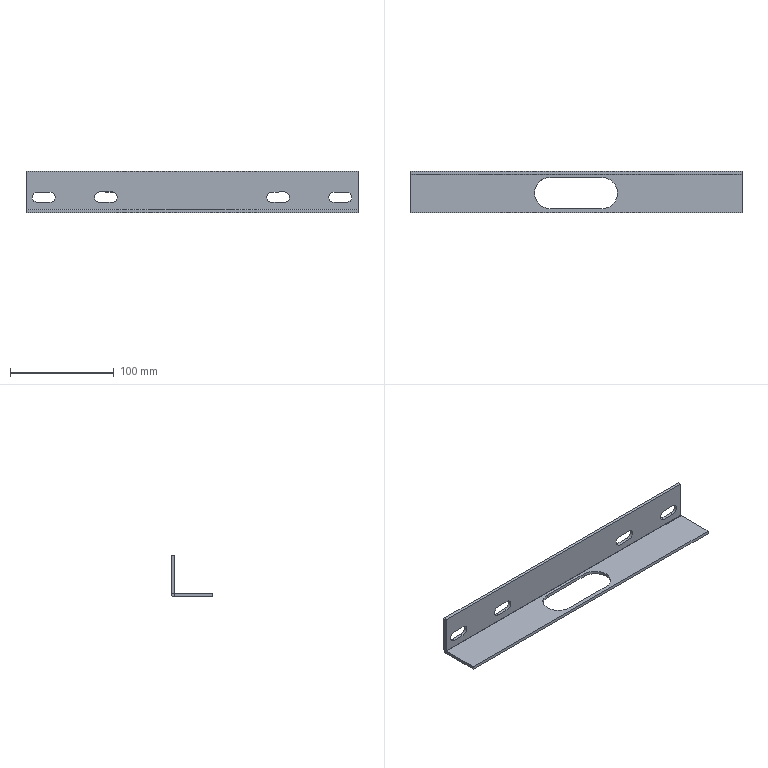Part | 1 solid | 35 faces | box 320 x 40 x 40 mm | volume 64216 mm3 | plane 22 | cylinder 13 | commonest cylinder face diameters 10 x8 30 x3 0.4 x1 6.4 x1
STEP:
#1=CARTESIAN_POINT('',(40.,-1.,-3.));
#2=VERTEX_POINT('',#1);
#3=CARTESIAN_POINT('',(25.,14.,-3.));
#4=VERTEX_POINT('',#3);
#5=CARTESIAN_POINT('',(25.,-1.,-3.));
#6=DIRECTION('',(0.,0.,1.));
#7=DIRECTION('',(1.,0.,0.));
#8=AXIS2_PLACEMENT_3D('',#5,#6,#7);
#9=CIRCLE('',#8,15.);
#10=EDGE_CURVE('',#2,#4,#9,.T.);
#11=ORIENTED_EDGE('',*,*,#10,.F.);
#12=CARTESIAN_POINT('',(40.,-1.,0.));
#13=VERTEX_POINT('',#12);
#14=CARTESIAN_POINT('',(40.,-1.,-10.));
#15=DIRECTION('',(0.,0.,1.));
#16=VECTOR('',#15,1000.);
#17=LINE('',#14,#16);
#18=EDGE_CURVE('',#2,#13,#17,.T.);
#19=ORIENTED_EDGE('',*,*,#18,.T.);
#20=CARTESIAN_POINT('',(25.,14.,0.));
#21=VERTEX_POINT('',#20);
#22=CARTESIAN_POINT('',(25.,-1.,0.));
#23=DIRECTION('',(0.,0.,1.));
#24=DIRECTION('',(1.,0.,0.));
#25=AXIS2_PLACEMENT_3D('',#22,#23,#24);
#26=CIRCLE('',#25,15.);
#27=EDGE_CURVE('',#13,#21,#26,.T.);
#28=ORIENTED_EDGE('',*,*,#27,.T.);
#29=CARTESIAN_POINT('',(25.,14.,-10.));
#30=DIRECTION('',(0.,0.,1.));
#31=VECTOR('',#30,1000.);
#32=LINE('',#29,#31);
#33=EDGE_CURVE('',#4,#21,#32,.T.);
#34=ORIENTED_EDGE('',*,*,#33,.F.);
#35=EDGE_LOOP('',(#11,#19,#28,#34));
#36=FACE_OUTER_BOUND('',#35,.T.);
#37=CARTESIAN_POINT('',(25.,-1.,-10.));
#38=DIRECTION('',(0.,0.,1.));
#39=DIRECTION('',(1.,0.,0.));
#40=AXIS2_PLACEMENT_3D('',#37,#38,#39);
#41=CYLINDRICAL_SURFACE('',#40,15.);
#42=ADVANCED_FACE('',(#36),#41,.F.);
#43=CARTESIAN_POINT('',(-160.,16.8,0.));
#44=VERTEX_POINT('',#43);
#45=CARTESIAN_POINT('',(-160.,-20.,0.));
#46=VERTEX_POINT('',#45);
#47=CARTESIAN_POINT('',(-160.,20.,0.));
#48=DIRECTION('',(0.,-1.,0.));
#49=VECTOR('',#48,1000.);
#50=LINE('',#47,#49);
#51=EDGE_CURVE('',#44,#46,#50,.T.);
#52=ORIENTED_EDGE('',*,*,#51,.F.);
#53=CARTESIAN_POINT('',(-160.,16.8,-3.));
#54=VERTEX_POINT('',#53);
#55=CARTESIAN_POINT('',(-160.,16.8,0.));
#56=DIRECTION('',(0.,0.,-1.));
#57=VECTOR('',#56,1000.);
#58=LINE('',#55,#57);
#59=EDGE_CURVE('',#44,#54,#58,.T.);
#60=ORIENTED_EDGE('',*,*,#59,.T.);
#61=CARTESIAN_POINT('',(-160.,-20.,-3.));
#62=VERTEX_POINT('',#61);
#63=CARTESIAN_POINT('',(-160.,20.,-3.));
#64=DIRECTION('',(0.,-1.,0.));
#65=VECTOR('',#64,1000.);
#66=LINE('',#63,#65);
#67=EDGE_CURVE('',#54,#62,#66,.T.);
#68=ORIENTED_EDGE('',*,*,#67,.T.);
#69=CARTESIAN_POINT('',(-160.,-20.,-3.));
#70=DIRECTION('',(0.,0.,1.));
#71=VECTOR('',#70,1000.);
#72=LINE('',#69,#71);
#73=EDGE_CURVE('',#62,#46,#72,.T.);
#74=ORIENTED_EDGE('',*,*,#73,.T.);
#75=EDGE_LOOP('',(#52,#60,#68,#74));
#76=FACE_OUTER_BOUND('',#75,.T.);
#77=CARTESIAN_POINT('',(-160.,20.,-3.));
#78=DIRECTION('',(-1.,0.,0.));
#79=DIRECTION('',(0.,0.,1.));
#80=AXIS2_PLACEMENT_3D('',#77,#78,#79);
#81=PLANE('',#80);
#82=ADVANCED_FACE('',(#76),#81,.T.);
#83=CARTESIAN_POINT('',(-25.,14.,-3.));
#84=VERTEX_POINT('',#83);
#85=CARTESIAN_POINT('',(0.,14.,-3.));
#86=DIRECTION('',(-1.,0.,0.));
#87=VECTOR('',#86,1000.);
#88=LINE('',#85,#87);
#89=EDGE_CURVE('',#4,#84,#88,.T.);
#90=ORIENTED_EDGE('',*,*,#89,.T.);
#91=CARTESIAN_POINT('',(-25.,-16.,-3.));
#92=VERTEX_POINT('',#91);
#93=CARTESIAN_POINT('',(-25.,-1.,-3.));
#94=DIRECTION('',(0.,0.,1.));
#95=DIRECTION('',(1.,0.,0.));
#96=AXIS2_PLACEMENT_3D('',#93,#94,#95);
#97=CIRCLE('',#96,15.);
#98=EDGE_CURVE('',#84,#92,#97,.T.);
#99=ORIENTED_EDGE('',*,*,#98,.T.);
#100=CARTESIAN_POINT('',(25.,-16.,-3.));
#101=VERTEX_POINT('',#100);
#102=CARTESIAN_POINT('',(0.,-16.,-3.));
#103=DIRECTION('',(1.,0.,0.));
#104=VECTOR('',#103,1000.);
#105=LINE('',#102,#104);
#106=EDGE_CURVE('',#92,#101,#105,.T.);
#107=ORIENTED_EDGE('',*,*,#106,.T.);
#108=CARTESIAN_POINT('',(25.,-1.,-3.));
#109=DIRECTION('',(0.,0.,1.));
#110=DIRECTION('',(1.,0.,0.));
#111=AXIS2_PLACEMENT_3D('',#108,#109,#110);
#112=CIRCLE('',#111,15.);
#113=EDGE_CURVE('',#101,#2,#112,.T.);
#114=ORIENTED_EDGE('',*,*,#113,.T.);
#115=ORIENTED_EDGE('',*,*,#10,.T.);
#116=EDGE_LOOP('',(#90,#99,#107,#114,#115));
#117=FACE_BOUND('',#116,.T.);
#118=CARTESIAN_POINT('',(160.,16.8,-3.));
#119=VERTEX_POINT('',#118);
#120=CARTESIAN_POINT('',(-160.,16.8,-3.));
#121=DIRECTION('',(1.,0.,0.));
#122=VECTOR('',#121,1000.);
#123=LINE('',#120,#122);
#124=EDGE_CURVE('',#54,#119,#123,.T.);
#125=ORIENTED_EDGE('',*,*,#124,.T.);
#126=CARTESIAN_POINT('',(160.,-20.,-3.));
#127=VERTEX_POINT('',#126);
#128=CARTESIAN_POINT('',(160.,20.,-3.));
#129=DIRECTION('',(0.,1.,0.));
#130=VECTOR('',#129,1000.);
#131=LINE('',#128,#130);
#132=EDGE_CURVE('',#127,#119,#131,.T.);
#133=ORIENTED_EDGE('',*,*,#132,.F.);
#134=CARTESIAN_POINT('',(-160.,-20.,-3.));
#135=DIRECTION('',(1.,0.,0.));
#136=VECTOR('',#135,1000.);
#137=LINE('',#134,#136);
#138=EDGE_CURVE('',#62,#127,#137,.T.);
#139=ORIENTED_EDGE('',*,*,#138,.F.);
#140=ORIENTED_EDGE('',*,*,#67,.F.);
#141=EDGE_LOOP('',(#125,#133,#139,#140));
#142=FACE_OUTER_BOUND('',#141,.T.);
#143=CARTESIAN_POINT('',(0.,0.,-3.));
#144=DIRECTION('',(0.,0.,1.));
#145=DIRECTION('',(1.,0.,0.));
#146=AXIS2_PLACEMENT_3D('',#143,#144,#145);
#147=PLANE('',#146);
#148=ADVANCED_FACE('',(#117,#142),#147,.F.);
#149=CARTESIAN_POINT('',(-25.,14.,0.));
#150=VERTEX_POINT('',#149);
#151=CARTESIAN_POINT('',(-25.,-16.,0.));
#152=VERTEX_POINT('',#151);
#153=CARTESIAN_POINT('',(-25.,-1.,0.));
#154=DIRECTION('',(0.,0.,1.));
#155=DIRECTION('',(1.,0.,0.));
#156=AXIS2_PLACEMENT_3D('',#153,#154,#155);
#157=CIRCLE('',#156,15.);
#158=EDGE_CURVE('',#150,#152,#157,.T.);
#159=ORIENTED_EDGE('',*,*,#158,.F.);
#160=CARTESIAN_POINT('',(-25.,14.,0.));
#161=DIRECTION('',(-1.,0.,0.));
#162=VECTOR('',#161,1000.);
#163=LINE('',#160,#162);
#164=EDGE_CURVE('',#21,#150,#163,.T.);
#165=ORIENTED_EDGE('',*,*,#164,.F.);
#166=ORIENTED_EDGE('',*,*,#27,.F.);
#167=CARTESIAN_POINT('',(25.,-16.,0.));
#168=VERTEX_POINT('',#167);
#169=CARTESIAN_POINT('',(25.,-1.,0.));
#170=DIRECTION('',(0.,0.,1.));
#171=DIRECTION('',(1.,0.,0.));
#172=AXIS2_PLACEMENT_3D('',#169,#170,#171);
#173=CIRCLE('',#172,15.);
#174=EDGE_CURVE('',#168,#13,#173,.T.);
#175=ORIENTED_EDGE('',*,*,#174,.F.);
#176=CARTESIAN_POINT('',(-25.,-16.,0.));
#177=DIRECTION('',(1.,0.,0.));
#178=VECTOR('',#177,1000.);
#179=LINE('',#176,#178);
#180=EDGE_CURVE('',#152,#168,#179,.T.);
#181=ORIENTED_EDGE('',*,*,#180,.F.);
#182=EDGE_LOOP('',(#159,#165,#166,#175,#181));
#183=FACE_BOUND('',#182,.T.);
#184=CARTESIAN_POINT('',(160.,-20.,0.));
#185=VERTEX_POINT('',#184);
#186=CARTESIAN_POINT('',(160.,16.8,0.));
#187=VERTEX_POINT('',#186);
#188=CARTESIAN_POINT('',(160.,20.,0.));
#189=DIRECTION('',(0.,1.,0.));
#190=VECTOR('',#189,1000.);
#191=LINE('',#188,#190);
#192=EDGE_CURVE('',#185,#187,#191,.T.);
#193=ORIENTED_EDGE('',*,*,#192,.T.);
#194=CARTESIAN_POINT('',(-160.,16.8,0.));
#195=DIRECTION('',(1.,0.,0.));
#196=VECTOR('',#195,1000.);
#197=LINE('',#194,#196);
#198=EDGE_CURVE('',#44,#187,#197,.T.);
#199=ORIENTED_EDGE('',*,*,#198,.F.);
#200=ORIENTED_EDGE('',*,*,#51,.T.);
#201=CARTESIAN_POINT('',(-160.,-20.,0.));
#202=DIRECTION('',(1.,0.,0.));
#203=VECTOR('',#202,1000.);
#204=LINE('',#201,#203);
#205=EDGE_CURVE('',#46,#185,#204,.T.);
#206=ORIENTED_EDGE('',*,*,#205,.T.);
#207=EDGE_LOOP('',(#193,#199,#200,#206));
#208=FACE_OUTER_BOUND('',#207,.T.);
#209=CARTESIAN_POINT('',(0.,0.,0.));
#210=DIRECTION('',(0.,0.,1.));
#211=DIRECTION('',(1.,0.,0.));
#212=AXIS2_PLACEMENT_3D('',#209,#210,#211);
#213=PLANE('',#212);
#214=ADVANCED_FACE('',(#183,#208),#213,.T.);
#215=CARTESIAN_POINT('',(160.,16.8,0.));
#216=DIRECTION('',(0.,0.,-1.));
#217=VECTOR('',#216,1000.);
#218=LINE('',#215,#217);
#219=EDGE_CURVE('',#187,#119,#218,.T.);
#220=ORIENTED_EDGE('',*,*,#219,.F.);
#221=ORIENTED_EDGE('',*,*,#192,.F.);
#222=CARTESIAN_POINT('',(160.,-20.,-3.));
#223=DIRECTION('',(0.,0.,1.));
#224=VECTOR('',#223,1000.);
#225=LINE('',#222,#224);
#226=EDGE_CURVE('',#127,#185,#225,.T.);
#227=ORIENTED_EDGE('',*,*,#226,.F.);
#228=ORIENTED_EDGE('',*,*,#132,.T.);
#229=EDGE_LOOP('',(#220,#221,#227,#228));
#230=FACE_OUTER_BOUND('',#229,.T.);
#231=CARTESIAN_POINT('',(160.,20.,-3.));
#232=DIRECTION('',(1.,0.,0.));
#233=DIRECTION('',(0.,0.,-1.));
#234=AXIS2_PLACEMENT_3D('',#231,#232,#233);
#235=PLANE('',#234);
#236=ADVANCED_FACE('',(#230),#235,.T.);
#237=ORIENTED_EDGE('',*,*,#205,.F.);
#238=ORIENTED_EDGE('',*,*,#73,.F.);
#239=ORIENTED_EDGE('',*,*,#138,.T.);
#240=ORIENTED_EDGE('',*,*,#226,.T.);
#241=EDGE_LOOP('',(#237,#238,#239,#240));
#242=FACE_OUTER_BOUND('',#241,.T.);
#243=CARTESIAN_POINT('',(-160.,-20.,-3.));
#244=DIRECTION('',(0.,-1.,0.));
#245=DIRECTION('',(0.,0.,-1.));
#246=AXIS2_PLACEMENT_3D('',#243,#244,#245);
#247=PLANE('',#246);
#248=ADVANCED_FACE('',(#242),#247,.T.);
#249=CARTESIAN_POINT('',(160.,17.,0.2));
#250=VERTEX_POINT('',#249);
#251=CARTESIAN_POINT('',(160.,20.,0.2));
#252=VERTEX_POINT('',#251);
#253=CARTESIAN_POINT('',(160.,20.,0.2));
#254=DIRECTION('',(0.,1.,0.));
#255=VECTOR('',#254,1000.);
#256=LINE('',#253,#255);
#257=EDGE_CURVE('',#250,#252,#256,.T.);
#258=ORIENTED_EDGE('',*,*,#257,.F.);
#259=CARTESIAN_POINT('',(160.,16.8,0.2));
#260=DIRECTION('',(1.,0.,0.));
#261=DIRECTION('',(0.,0.,1.));
#262=AXIS2_PLACEMENT_3D('',#259,#260,#261);
#263=CIRCLE('',#262,0.2);
#264=EDGE_CURVE('',#187,#250,#263,.T.);
#265=ORIENTED_EDGE('',*,*,#264,.F.);
#266=ORIENTED_EDGE('',*,*,#219,.T.);
#267=CARTESIAN_POINT('',(160.,16.8,0.2));
#268=DIRECTION('',(1.,0.,0.));
#269=DIRECTION('',(0.,0.,1.));
#270=AXIS2_PLACEMENT_3D('',#267,#268,#269);
#271=CIRCLE('',#270,3.2);
#272=EDGE_CURVE('',#119,#252,#271,.T.);
#273=ORIENTED_EDGE('',*,*,#272,.T.);
#274=EDGE_LOOP('',(#258,#265,#266,#273));
#275=FACE_OUTER_BOUND('',#274,.T.);
#276=CARTESIAN_POINT('',(160.,16.8,0.2));
#277=DIRECTION('',(1.,0.,0.));
#278=DIRECTION('',(0.,0.,-1.));
#279=AXIS2_PLACEMENT_3D('',#276,#277,#278);
#280=PLANE('',#279);
#281=ADVANCED_FACE('',(#275),#280,.T.);
#282=CARTESIAN_POINT('',(-160.,17.,0.2));
#283=VERTEX_POINT('',#282);
#284=CARTESIAN_POINT('',(-160.,16.8,0.2));
#285=DIRECTION('',(-1.,0.,0.));
#286=DIRECTION('',(0.,0.,1.));
#287=AXIS2_PLACEMENT_3D('',#284,#285,#286);
#288=CIRCLE('',#287,0.2);
#289=EDGE_CURVE('',#283,#44,#288,.T.);
#290=ORIENTED_EDGE('',*,*,#289,.F.);
#291=CARTESIAN_POINT('',(-160.,20.,0.2));
#292=VERTEX_POINT('',#291);
#293=CARTESIAN_POINT('',(-160.,17.,0.2));
#294=DIRECTION('',(0.,1.,0.));
#295=VECTOR('',#294,1000.);
#296=LINE('',#293,#295);
#297=EDGE_CURVE('',#283,#292,#296,.T.);
#298=ORIENTED_EDGE('',*,*,#297,.T.);
#299=CARTESIAN_POINT('',(-160.,16.8,0.2));
#300=DIRECTION('',(-1.,0.,0.));
#301=DIRECTION('',(0.,0.,1.));
#302=AXIS2_PLACEMENT_3D('',#299,#300,#301);
#303=CIRCLE('',#302,3.2);
#304=EDGE_CURVE('',#292,#54,#303,.T.);
#305=ORIENTED_EDGE('',*,*,#304,.T.);
#306=ORIENTED_EDGE('',*,*,#59,.F.);
#307=EDGE_LOOP('',(#290,#298,#305,#306));
#308=FACE_OUTER_BOUND('',#307,.T.);
#309=CARTESIAN_POINT('',(-160.,16.8,0.2));
#310=DIRECTION('',(1.,0.,0.));
#311=DIRECTION('',(0.,0.,-1.));
#312=AXIS2_PLACEMENT_3D('',#309,#310,#311);
#313=PLANE('',#312);
#314=ADVANCED_FACE('',(#308),#313,.F.);
#315=ORIENTED_EDGE('',*,*,#124,.F.);
#316=ORIENTED_EDGE('',*,*,#304,.F.);
#317=CARTESIAN_POINT('',(160.,20.,0.2));
#318=DIRECTION('',(1.,0.,0.));
#319=VECTOR('',#318,1000.);
#320=LINE('',#317,#319);
#321=EDGE_CURVE('',#292,#252,#320,.T.);
#322=ORIENTED_EDGE('',*,*,#321,.T.);
#323=ORIENTED_EDGE('',*,*,#272,.F.);
#324=EDGE_LOOP('',(#315,#316,#322,#323));
#325=FACE_OUTER_BOUND('',#324,.T.);
#326=CARTESIAN_POINT('',(-160.,16.8,0.2));
#327=DIRECTION('',(-1.,0.,0.));
#328=DIRECTION('',(0.,1.,0.));
#329=AXIS2_PLACEMENT_3D('',#326,#327,#328);
#330=CYLINDRICAL_SURFACE('',#329,3.2);
#331=ADVANCED_FACE('',(#325),#330,.T.);
#332=ORIENTED_EDGE('',*,*,#198,.T.);
#333=ORIENTED_EDGE('',*,*,#264,.T.);
#334=CARTESIAN_POINT('',(160.,17.,0.2));
#335=DIRECTION('',(-1.,0.,0.));
#336=VECTOR('',#335,1000.);
#337=LINE('',#334,#336);
#338=EDGE_CURVE('',#250,#283,#337,.T.);
#339=ORIENTED_EDGE('',*,*,#338,.T.);
#340=ORIENTED_EDGE('',*,*,#289,.T.);
#341=EDGE_LOOP('',(#332,#333,#339,#340));
#342=FACE_OUTER_BOUND('',#341,.T.);
#343=CARTESIAN_POINT('',(-160.,16.8,0.2));
#344=DIRECTION('',(-1.,0.,0.));
#345=DIRECTION('',(0.,1.,0.));
#346=AXIS2_PLACEMENT_3D('',#343,#344,#345);
#347=CYLINDRICAL_SURFACE('',#346,0.2);
#348=ADVANCED_FACE('',(#342),#347,.F.);
#349=ORIENTED_EDGE('',*,*,#257,.T.);
#350=CARTESIAN_POINT('',(160.,20.,37.));
#351=VERTEX_POINT('',#350);
#352=CARTESIAN_POINT('',(160.,20.,0.));
#353=DIRECTION('',(0.,0.,-1.));
#354=VECTOR('',#353,1000.);
#355=LINE('',#352,#354);
#356=EDGE_CURVE('',#351,#252,#355,.T.);
#357=ORIENTED_EDGE('',*,*,#356,.F.);
#358=CARTESIAN_POINT('',(160.,17.,37.));
#359=VERTEX_POINT('',#358);
#360=CARTESIAN_POINT('',(160.,20.,37.));
#361=DIRECTION('',(0.,-1.,0.));
#362=VECTOR('',#361,1000.);
#363=LINE('',#360,#362);
#364=EDGE_CURVE('',#351,#359,#363,.T.);
#365=ORIENTED_EDGE('',*,*,#364,.T.);
#366=CARTESIAN_POINT('',(160.,17.,0.));
#367=DIRECTION('',(0.,0.,-1.));
#368=VECTOR('',#367,1000.);
#369=LINE('',#366,#368);
#370=EDGE_CURVE('',#359,#250,#369,.T.);
#371=ORIENTED_EDGE('',*,*,#370,.T.);
#372=EDGE_LOOP('',(#349,#357,#365,#371));
#373=FACE_OUTER_BOUND('',#372,.T.);
#374=CARTESIAN_POINT('',(160.,20.,0.));
#375=DIRECTION('',(-1.,0.,0.));
#376=DIRECTION('',(0.,0.,1.));
#377=AXIS2_PLACEMENT_3D('',#374,#375,#376);
#378=PLANE('',#377);
#379=ADVANCED_FACE('',(#373),#378,.F.);
#380=ORIENTED_EDGE('',*,*,#297,.F.);
#381=CARTESIAN_POINT('',(-160.,17.,37.));
#382=VERTEX_POINT('',#381);
#383=CARTESIAN_POINT('',(-160.,17.,37.));
#384=DIRECTION('',(0.,0.,1.));
#385=VECTOR('',#384,1000.);
#386=LINE('',#383,#385);
#387=EDGE_CURVE('',#283,#382,#386,.T.);
#388=ORIENTED_EDGE('',*,*,#387,.T.);
#389=CARTESIAN_POINT('',(-160.,20.,37.));
#390=VERTEX_POINT('',#389);
#391=CARTESIAN_POINT('',(-160.,20.,37.));
#392=DIRECTION('',(0.,-1.,0.));
#393=VECTOR('',#392,1000.);
#394=LINE('',#391,#393);
#395=EDGE_CURVE('',#390,#382,#394,.T.);
#396=ORIENTED_EDGE('',*,*,#395,.F.);
#397=CARTESIAN_POINT('',(-160.,20.,0.));
#398=DIRECTION('',(0.,0.,1.));
#399=VECTOR('',#398,1000.);
#400=LINE('',#397,#399);
#401=EDGE_CURVE('',#292,#390,#400,.T.);
#402=ORIENTED_EDGE('',*,*,#401,.F.);
#403=EDGE_LOOP('',(#380,#388,#396,#402));
#404=FACE_OUTER_BOUND('',#403,.T.);
#405=CARTESIAN_POINT('',(-160.,20.,37.));
#406=DIRECTION('',(1.,0.,0.));
#407=DIRECTION('',(0.,0.,-1.));
#408=AXIS2_PLACEMENT_3D('',#405,#406,#407);
#409=PLANE('',#408);
#410=ADVANCED_FACE('',(#404),#409,.F.);
#411=CARTESIAN_POINT('',(-149.,20.,17.));
#412=VERTEX_POINT('',#411);
#413=CARTESIAN_POINT('',(-137.,20.,17.));
#414=VERTEX_POINT('',#413);
#415=CARTESIAN_POINT('',(-149.,20.,17.));
#416=DIRECTION('',(1.,0.,0.));
#417=VECTOR('',#416,1000.);
#418=LINE('',#415,#417);
#419=EDGE_CURVE('',#412,#414,#418,.T.);
#420=ORIENTED_EDGE('',*,*,#419,.F.);
#421=CARTESIAN_POINT('',(-149.,20.,7.));
#422=VERTEX_POINT('',#421);
#423=CARTESIAN_POINT('',(-149.,20.,12.));
#424=DIRECTION('',(0.,1.,0.));
#425=DIRECTION('',(0.,0.,1.));
#426=AXIS2_PLACEMENT_3D('',#423,#424,#425);
#427=CIRCLE('',#426,5.);
#428=EDGE_CURVE('',#422,#412,#427,.T.);
#429=ORIENTED_EDGE('',*,*,#428,.F.);
#430=CARTESIAN_POINT('',(-137.,20.,7.));
#431=VERTEX_POINT('',#430);
#432=CARTESIAN_POINT('',(-149.,20.,7.));
#433=DIRECTION('',(-1.,0.,0.));
#434=VECTOR('',#433,1000.);
#435=LINE('',#432,#434);
#436=EDGE_CURVE('',#431,#422,#435,.T.);
#437=ORIENTED_EDGE('',*,*,#436,.F.);
#438=CARTESIAN_POINT('',(-137.,20.,12.));
#439=DIRECTION('',(0.,1.,0.));
#440=DIRECTION('',(0.,0.,1.));
#441=AXIS2_PLACEMENT_3D('',#438,#439,#440);
#442=CIRCLE('',#441,5.);
#443=EDGE_CURVE('',#414,#431,#442,.T.);
#444=ORIENTED_EDGE('',*,*,#443,.F.);
#445=EDGE_LOOP('',(#420,#429,#437,#444));
#446=FACE_BOUND('',#445,.T.);
#447=CARTESIAN_POINT('',(-89.,20.,17.));
#448=VERTEX_POINT('',#447);
#449=CARTESIAN_POINT('',(-77.,20.,17.));
#450=VERTEX_POINT('',#449);
#451=CARTESIAN_POINT('',(-89.,20.,17.));
#452=DIRECTION('',(1.,0.,0.));
#453=VECTOR('',#452,1000.);
#454=LINE('',#451,#453);
#455=EDGE_CURVE('',#448,#450,#454,.T.);
#456=ORIENTED_EDGE('',*,*,#455,.F.);
#457=CARTESIAN_POINT('',(-89.,20.,7.));
#458=VERTEX_POINT('',#457);
#459=CARTESIAN_POINT('',(-89.,20.,12.));
#460=DIRECTION('',(0.,1.,0.));
#461=DIRECTION('',(0.,0.,1.));
#462=AXIS2_PLACEMENT_3D('',#459,#460,#461);
#463=CIRCLE('',#462,5.);
#464=EDGE_CURVE('',#458,#448,#463,.T.);
#465=ORIENTED_EDGE('',*,*,#464,.F.);
#466=CARTESIAN_POINT('',(-77.,20.,7.));
#467=VERTEX_POINT('',#466);
#468=CARTESIAN_POINT('',(-89.,20.,7.));
#469=DIRECTION('',(-1.,0.,0.));
#470=VECTOR('',#469,1000.);
#471=LINE('',#468,#470);
#472=EDGE_CURVE('',#467,#458,#471,.T.);
#473=ORIENTED_EDGE('',*,*,#472,.F.);
#474=CARTESIAN_POINT('',(-77.,20.,12.));
#475=DIRECTION('',(0.,1.,0.));
#476=DIRECTION('',(0.,0.,1.));
#477=AXIS2_PLACEMENT_3D('',#474,#475,#476);
#478=CIRCLE('',#477,5.);
#479=EDGE_CURVE('',#450,#467,#478,.T.);
#480=ORIENTED_EDGE('',*,*,#479,.F.);
#481=EDGE_LOOP('',(#456,#465,#473,#480));
#482=FACE_BOUND('',#481,.T.);
#483=CARTESIAN_POINT('',(89.,20.,7.));
#484=VERTEX_POINT('',#483);
#485=CARTESIAN_POINT('',(77.,20.,7.));
#486=VERTEX_POINT('',#485);
#487=CARTESIAN_POINT('',(89.,20.,7.));
#488=DIRECTION('',(-1.,0.,0.));
#489=VECTOR('',#488,1000.);
#490=LINE('',#487,#489);
#491=EDGE_CURVE('',#484,#486,#490,.T.);
#492=ORIENTED_EDGE('',*,*,#491,.F.);
#493=CARTESIAN_POINT('',(89.,20.,17.));
#494=VERTEX_POINT('',#493);
#495=CARTESIAN_POINT('',(89.,20.,12.));
#496=DIRECTION('',(0.,1.,0.));
#497=DIRECTION('',(0.,0.,-1.));
#498=AXIS2_PLACEMENT_3D('',#495,#496,#497);
#499=CIRCLE('',#498,5.);
#500=EDGE_CURVE('',#494,#484,#499,.T.);
#501=ORIENTED_EDGE('',*,*,#500,.F.);
#502=CARTESIAN_POINT('',(77.,20.,17.));
#503=VERTEX_POINT('',#502);
#504=CARTESIAN_POINT('',(89.,20.,17.));
#505=DIRECTION('',(1.,0.,0.));
#506=VECTOR('',#505,1000.);
#507=LINE('',#504,#506);
#508=EDGE_CURVE('',#503,#494,#507,.T.);
#509=ORIENTED_EDGE('',*,*,#508,.F.);
#510=CARTESIAN_POINT('',(77.,20.,12.));
#511=DIRECTION('',(0.,1.,0.));
#512=DIRECTION('',(0.,0.,-1.));
#513=AXIS2_PLACEMENT_3D('',#510,#511,#512);
#514=CIRCLE('',#513,5.);
#515=EDGE_CURVE('',#486,#503,#514,.T.);
#516=ORIENTED_EDGE('',*,*,#515,.F.);
#517=EDGE_LOOP('',(#492,#501,#509,#516));
#518=FACE_BOUND('',#517,.T.);
#519=CARTESIAN_POINT('',(149.,20.,7.));
#520=VERTEX_POINT('',#519);
#521=CARTESIAN_POINT('',(137.,20.,7.));
#522=VERTEX_POINT('',#521);
#523=CARTESIAN_POINT('',(149.,20.,7.));
#524=DIRECTION('',(-1.,0.,0.));
#525=VECTOR('',#524,1000.);
#526=LINE('',#523,#525);
#527=EDGE_CURVE('',#520,#522,#526,.T.);
#528=ORIENTED_EDGE('',*,*,#527,.F.);
#529=CARTESIAN_POINT('',(149.,20.,17.));
#530=VERTEX_POINT('',#529);
#531=CARTESIAN_POINT('',(149.,20.,12.));
#532=DIRECTION('',(0.,1.,0.));
#533=DIRECTION('',(0.,0.,-1.));
#534=AXIS2_PLACEMENT_3D('',#531,#532,#533);
#535=CIRCLE('',#534,5.);
#536=EDGE_CURVE('',#530,#520,#535,.T.);
#537=ORIENTED_EDGE('',*,*,#536,.F.);
#538=CARTESIAN_POINT('',(137.,20.,17.));
#539=VERTEX_POINT('',#538);
#540=CARTESIAN_POINT('',(149.,20.,17.));
#541=DIRECTION('',(1.,0.,0.));
#542=VECTOR('',#541,1000.);
#543=LINE('',#540,#542);
#544=EDGE_CURVE('',#539,#530,#543,.T.);
#545=ORIENTED_EDGE('',*,*,#544,.F.);
#546=CARTESIAN_POINT('',(137.,20.,12.));
#547=DIRECTION('',(0.,1.,0.));
#548=DIRECTION('',(0.,0.,-1.));
#549=AXIS2_PLACEMENT_3D('',#546,#547,#548);
#550=CIRCLE('',#549,5.);
#551=EDGE_CURVE('',#522,#539,#550,.T.);
#552=ORIENTED_EDGE('',*,*,#551,.F.);
#553=EDGE_LOOP('',(#528,#537,#545,#552));
#554=FACE_BOUND('',#553,.T.);
#555=ORIENTED_EDGE('',*,*,#321,.F.);
#556=ORIENTED_EDGE('',*,*,#401,.T.);
#557=CARTESIAN_POINT('',(0.,20.,37.));
#558=DIRECTION('',(1.,0.,0.));
#559=VECTOR('',#558,1000.);
#560=LINE('',#557,#559);
#561=EDGE_CURVE('',#390,#351,#560,.T.);
#562=ORIENTED_EDGE('',*,*,#561,.T.);
#563=ORIENTED_EDGE('',*,*,#356,.T.);
#564=EDGE_LOOP('',(#555,#556,#562,#563));
#565=FACE_OUTER_BOUND('',#564,.T.);
#566=CARTESIAN_POINT('',(0.,20.,0.));
#567=DIRECTION('',(0.,-1.,0.));
#568=DIRECTION('',(0.,0.,-1.));
#569=AXIS2_PLACEMENT_3D('',#566,#567,#568);
#570=PLANE('',#569);
#571=ADVANCED_FACE('',(#446,#482,#518,#554,#565),#570,.F.);
#572=CARTESIAN_POINT('',(-149.,17.,17.));
#573=VERTEX_POINT('',#572);
#574=CARTESIAN_POINT('',(-149.,17.,7.));
#575=VERTEX_POINT('',#574);
#576=CARTESIAN_POINT('',(-149.,17.,12.));
#577=DIRECTION('',(0.,-1.,0.));
#578=DIRECTION('',(0.,0.,-1.));
#579=AXIS2_PLACEMENT_3D('',#576,#577,#578);
#580=CIRCLE('',#579,5.);
#581=EDGE_CURVE('',#573,#575,#580,.T.);
#582=ORIENTED_EDGE('',*,*,#581,.F.);
#583=CARTESIAN_POINT('',(-137.,17.,17.));
#584=VERTEX_POINT('',#583);
#585=CARTESIAN_POINT('',(0.,17.,17.));
#586=DIRECTION('',(-1.,0.,0.));
#587=VECTOR('',#586,1000.);
#588=LINE('',#585,#587);
#589=EDGE_CURVE('',#584,#573,#588,.T.);
#590=ORIENTED_EDGE('',*,*,#589,.F.);
#591=CARTESIAN_POINT('',(-137.,17.,7.));
#592=VERTEX_POINT('',#591);
#593=CARTESIAN_POINT('',(-137.,17.,12.));
#594=DIRECTION('',(0.,-1.,0.));
#595=DIRECTION('',(0.,0.,-1.));
#596=AXIS2_PLACEMENT_3D('',#593,#594,#595);
#597=CIRCLE('',#596,5.);
#598=EDGE_CURVE('',#592,#584,#597,.T.);
#599=ORIENTED_EDGE('',*,*,#598,.F.);
#600=CARTESIAN_POINT('',(0.,17.,7.));
#601=DIRECTION('',(1.,0.,0.));
#602=VECTOR('',#601,1000.);
#603=LINE('',#600,#602);
#604=EDGE_CURVE('',#575,#592,#603,.T.);
#605=ORIENTED_EDGE('',*,*,#604,.F.);
#606=EDGE_LOOP('',(#582,#590,#599,#605));
#607=FACE_BOUND('',#606,.T.);
#608=CARTESIAN_POINT('',(-89.,17.,17.));
#609=VERTEX_POINT('',#608);
#610=CARTESIAN_POINT('',(-89.,17.,7.));
#611=VERTEX_POINT('',#610);
#612=CARTESIAN_POINT('',(-89.,17.,12.));
#613=DIRECTION('',(0.,-1.,0.));
#614=DIRECTION('',(0.,0.,-1.));
#615=AXIS2_PLACEMENT_3D('',#612,#613,#614);
#616=CIRCLE('',#615,5.);
#617=EDGE_CURVE('',#609,#611,#616,.T.);
#618=ORIENTED_EDGE('',*,*,#617,.F.);
#619=CARTESIAN_POINT('',(-77.,17.,17.));
#620=VERTEX_POINT('',#619);
#621=CARTESIAN_POINT('',(0.,17.,17.));
#622=DIRECTION('',(-1.,0.,0.));
#623=VECTOR('',#622,1000.);
#624=LINE('',#621,#623);
#625=EDGE_CURVE('',#620,#609,#624,.T.);
#626=ORIENTED_EDGE('',*,*,#625,.F.);
#627=CARTESIAN_POINT('',(-77.,17.,7.));
#628=VERTEX_POINT('',#627);
#629=CARTESIAN_POINT('',(-77.,17.,12.));
#630=DIRECTION('',(0.,-1.,0.));
#631=DIRECTION('',(0.,0.,-1.));
#632=AXIS2_PLACEMENT_3D('',#629,#630,#631);
#633=CIRCLE('',#632,5.);
#634=EDGE_CURVE('',#628,#620,#633,.T.);
#635=ORIENTED_EDGE('',*,*,#634,.F.);
#636=CARTESIAN_POINT('',(0.,17.,7.));
#637=DIRECTION('',(1.,0.,0.));
#638=VECTOR('',#637,1000.);
#639=LINE('',#636,#638);
#640=EDGE_CURVE('',#611,#628,#639,.T.);
#641=ORIENTED_EDGE('',*,*,#640,.F.);
#642=EDGE_LOOP('',(#618,#626,#635,#641));
#643=FACE_BOUND('',#642,.T.);
#644=CARTESIAN_POINT('',(89.,17.,7.));
#645=VERTEX_POINT('',#644);
#646=CARTESIAN_POINT('',(89.,17.,17.));
#647=VERTEX_POINT('',#646);
#648=CARTESIAN_POINT('',(89.,17.,12.));
#649=DIRECTION('',(0.,-1.,0.));
#650=DIRECTION('',(0.,0.,-1.));
#651=AXIS2_PLACEMENT_3D('',#648,#649,#650);
#652=CIRCLE('',#651,5.);
#653=EDGE_CURVE('',#645,#647,#652,.T.);
#654=ORIENTED_EDGE('',*,*,#653,.F.);
#655=CARTESIAN_POINT('',(77.,17.,7.));
#656=VERTEX_POINT('',#655);
#657=CARTESIAN_POINT('',(0.,17.,7.));
#658=DIRECTION('',(1.,0.,0.));
#659=VECTOR('',#658,1000.);
#660=LINE('',#657,#659);
#661=EDGE_CURVE('',#656,#645,#660,.T.);
#662=ORIENTED_EDGE('',*,*,#661,.F.);
#663=CARTESIAN_POINT('',(77.,17.,17.));
#664=VERTEX_POINT('',#663);
#665=CARTESIAN_POINT('',(77.,17.,12.));
#666=DIRECTION('',(0.,-1.,0.));
#667=DIRECTION('',(0.,0.,-1.));
#668=AXIS2_PLACEMENT_3D('',#665,#666,#667);
#669=CIRCLE('',#668,5.);
#670=EDGE_CURVE('',#664,#656,#669,.T.);
#671=ORIENTED_EDGE('',*,*,#670,.F.);
#672=CARTESIAN_POINT('',(0.,17.,17.));
#673=DIRECTION('',(-1.,0.,0.));
#674=VECTOR('',#673,1000.);
#675=LINE('',#672,#674);
#676=EDGE_CURVE('',#647,#664,#675,.T.);
#677=ORIENTED_EDGE('',*,*,#676,.F.);
#678=EDGE_LOOP('',(#654,#662,#671,#677));
#679=FACE_BOUND('',#678,.T.);
#680=CARTESIAN_POINT('',(149.,17.,7.));
#681=VERTEX_POINT('',#680);
#682=CARTESIAN_POINT('',(149.,17.,17.));
#683=VERTEX_POINT('',#682);
#684=CARTESIAN_POINT('',(149.,17.,12.));
#685=DIRECTION('',(0.,-1.,0.));
#686=DIRECTION('',(0.,0.,-1.));
#687=AXIS2_PLACEMENT_3D('',#684,#685,#686);
#688=CIRCLE('',#687,5.);
#689=EDGE_CURVE('',#681,#683,#688,.T.);
#690=ORIENTED_EDGE('',*,*,#689,.F.);
#691=CARTESIAN_POINT('',(137.,17.,7.));
#692=VERTEX_POINT('',#691);
#693=CARTESIAN_POINT('',(0.,17.,7.));
#694=DIRECTION('',(1.,0.,0.));
#695=VECTOR('',#694,1000.);
#696=LINE('',#693,#695);
#697=EDGE_CURVE('',#692,#681,#696,.T.);
#698=ORIENTED_EDGE('',*,*,#697,.F.);
#699=CARTESIAN_POINT('',(137.,17.,17.));
#700=VERTEX_POINT('',#699);
#701=CARTESIAN_POINT('',(137.,17.,12.));
#702=DIRECTION('',(0.,-1.,0.));
#703=DIRECTION('',(0.,0.,-1.));
#704=AXIS2_PLACEMENT_3D('',#701,#702,#703);
#705=CIRCLE('',#704,5.);
#706=EDGE_CURVE('',#700,#692,#705,.T.);
#707=ORIENTED_EDGE('',*,*,#706,.F.);
#708=CARTESIAN_POINT('',(0.,17.,17.));
#709=DIRECTION('',(-1.,0.,0.));
#710=VECTOR('',#709,1000.);
#711=LINE('',#708,#710);
#712=EDGE_CURVE('',#683,#700,#711,.T.);
#713=ORIENTED_EDGE('',*,*,#712,.F.);
#714=EDGE_LOOP('',(#690,#698,#707,#713));
#715=FACE_BOUND('',#714,.T.);
#716=ORIENTED_EDGE('',*,*,#387,.F.);
#717=ORIENTED_EDGE('',*,*,#338,.F.);
#718=ORIENTED_EDGE('',*,*,#370,.F.);
#719=CARTESIAN_POINT('',(160.,17.,37.));
#720=DIRECTION('',(1.,0.,0.));
#721=VECTOR('',#720,1000.);
#722=LINE('',#719,#721);
#723=EDGE_CURVE('',#382,#359,#722,.T.);
#724=ORIENTED_EDGE('',*,*,#723,.F.);
#725=EDGE_LOOP('',(#716,#717,#718,#724));
#726=FACE_OUTER_BOUND('',#725,.T.);
#727=CARTESIAN_POINT('',(0.,17.,0.));
#728=DIRECTION('',(0.,-1.,0.));
#729=DIRECTION('',(0.,0.,-1.));
#730=AXIS2_PLACEMENT_3D('',#727,#728,#729);
#731=PLANE('',#730);
#732=ADVANCED_FACE('',(#607,#643,#679,#715,#726),#731,.T.);
#733=ORIENTED_EDGE('',*,*,#723,.T.);
#734=ORIENTED_EDGE('',*,*,#364,.F.);
#735=ORIENTED_EDGE('',*,*,#561,.F.);
#736=ORIENTED_EDGE('',*,*,#395,.T.);
#737=EDGE_LOOP('',(#733,#734,#735,#736));
#738=FACE_OUTER_BOUND('',#737,.T.);
#739=CARTESIAN_POINT('',(160.,20.,37.));
#740=DIRECTION('',(0.,0.,-1.));
#741=DIRECTION('',(0.,1.,0.));
#742=AXIS2_PLACEMENT_3D('',#739,#740,#741);
#743=PLANE('',#742);
#744=ADVANCED_FACE('',(#738),#743,.F.);
#745=CARTESIAN_POINT('',(-25.,14.,-10.));
#746=DIRECTION('',(0.,0.,1.));
#747=VECTOR('',#746,1000.);
#748=LINE('',#745,#747);
#749=EDGE_CURVE('',#84,#150,#748,.T.);
#750=ORIENTED_EDGE('',*,*,#749,.T.);
#751=ORIENTED_EDGE('',*,*,#158,.T.);
#752=CARTESIAN_POINT('',(-25.,-16.,-10.));
#753=DIRECTION('',(0.,0.,1.));
#754=VECTOR('',#753,1000.);
#755=LINE('',#752,#754);
#756=EDGE_CURVE('',#92,#152,#755,.T.);
#757=ORIENTED_EDGE('',*,*,#756,.F.);
#758=ORIENTED_EDGE('',*,*,#98,.F.);
#759=EDGE_LOOP('',(#750,#751,#757,#758));
#760=FACE_OUTER_BOUND('',#759,.T.);
#761=CARTESIAN_POINT('',(-25.,-1.,-10.));
#762=DIRECTION('',(0.,0.,1.));
#763=DIRECTION('',(1.,0.,0.));
#764=AXIS2_PLACEMENT_3D('',#761,#762,#763);
#765=CYLINDRICAL_SURFACE('',#764,15.);
#766=ADVANCED_FACE('',(#760),#765,.F.);
#767=ORIENTED_EDGE('',*,*,#33,.T.);
#768=ORIENTED_EDGE('',*,*,#164,.T.);
#769=ORIENTED_EDGE('',*,*,#749,.F.);
#770=ORIENTED_EDGE('',*,*,#89,.F.);
#771=EDGE_LOOP('',(#767,#768,#769,#770));
#772=FACE_OUTER_BOUND('',#771,.T.);
#773=CARTESIAN_POINT('',(-25.,14.,-10.));
#774=DIRECTION('',(0.,1.,0.));
#775=DIRECTION('',(-1.,0.,0.));
#776=AXIS2_PLACEMENT_3D('',#773,#774,#775);
#777=PLANE('',#776);
#778=ADVANCED_FACE('',(#772),#777,.F.);
#779=ORIENTED_EDGE('',*,*,#18,.F.);
#780=ORIENTED_EDGE('',*,*,#113,.F.);
#781=CARTESIAN_POINT('',(25.,-16.,-10.));
#782=DIRECTION('',(0.,0.,1.));
#783=VECTOR('',#782,1000.);
#784=LINE('',#781,#783);
#785=EDGE_CURVE('',#101,#168,#784,.T.);
#786=ORIENTED_EDGE('',*,*,#785,.T.);
#787=ORIENTED_EDGE('',*,*,#174,.T.);
#788=EDGE_LOOP('',(#779,#780,#786,#787));
#789=FACE_OUTER_BOUND('',#788,.T.);
#790=CARTESIAN_POINT('',(25.,-1.,-10.));
#791=DIRECTION('',(0.,0.,1.));
#792=DIRECTION('',(1.,0.,0.));
#793=AXIS2_PLACEMENT_3D('',#790,#791,#792);
#794=CYLINDRICAL_SURFACE('',#793,15.);
#795=ADVANCED_FACE('',(#789),#794,.F.);
#796=ORIENTED_EDGE('',*,*,#756,.T.);
#797=ORIENTED_EDGE('',*,*,#180,.T.);
#798=ORIENTED_EDGE('',*,*,#785,.F.);
#799=ORIENTED_EDGE('',*,*,#106,.F.);
#800=EDGE_LOOP('',(#796,#797,#798,#799));
#801=FACE_OUTER_BOUND('',#800,.T.);
#802=CARTESIAN_POINT('',(-25.,-16.,-10.));
#803=DIRECTION('',(0.,-1.,0.));
#804=DIRECTION('',(1.,0.,0.));
#805=AXIS2_PLACEMENT_3D('',#802,#803,#804);
#806=PLANE('',#805);
#807=ADVANCED_FACE('',(#801),#806,.F.);
#808=ORIENTED_EDGE('',*,*,#689,.T.);
#809=CARTESIAN_POINT('',(149.,10.,17.));
#810=DIRECTION('',(0.,1.,0.));
#811=VECTOR('',#810,1000.);
#812=LINE('',#809,#811);
#813=EDGE_CURVE('',#683,#530,#812,.T.);
#814=ORIENTED_EDGE('',*,*,#813,.T.);
#815=ORIENTED_EDGE('',*,*,#536,.T.);
#816=CARTESIAN_POINT('',(149.,10.,7.));
#817=DIRECTION('',(0.,1.,0.));
#818=VECTOR('',#817,1000.);
#819=LINE('',#816,#818);
#820=EDGE_CURVE('',#681,#520,#819,.T.);
#821=ORIENTED_EDGE('',*,*,#820,.F.);
#822=EDGE_LOOP('',(#808,#814,#815,#821));
#823=FACE_OUTER_BOUND('',#822,.T.);
#824=CARTESIAN_POINT('',(149.,10.,12.));
#825=DIRECTION('',(0.,1.,0.));
#826=DIRECTION('',(0.,0.,1.));
#827=AXIS2_PLACEMENT_3D('',#824,#825,#826);
#828=CYLINDRICAL_SURFACE('',#827,5.);
#829=ADVANCED_FACE('',(#823),#828,.F.);
#830=ORIENTED_EDGE('',*,*,#712,.T.);
#831=CARTESIAN_POINT('',(137.,10.,17.));
#832=DIRECTION('',(0.,1.,0.));
#833=VECTOR('',#832,1000.);
#834=LINE('',#831,#833);
#835=EDGE_CURVE('',#700,#539,#834,.T.);
#836=ORIENTED_EDGE('',*,*,#835,.T.);
#837=ORIENTED_EDGE('',*,*,#544,.T.);
#838=ORIENTED_EDGE('',*,*,#813,.F.);
#839=EDGE_LOOP('',(#830,#836,#837,#838));
#840=FACE_OUTER_BOUND('',#839,.T.);
#841=CARTESIAN_POINT('',(149.,10.,17.));
#842=DIRECTION('',(0.,0.,1.));
#843=DIRECTION('',(0.,-1.,0.));
#844=AXIS2_PLACEMENT_3D('',#841,#842,#843);
#845=PLANE('',#844);
#846=ADVANCED_FACE('',(#840),#845,.F.);
#847=ORIENTED_EDGE('',*,*,#706,.T.);
#848=CARTESIAN_POINT('',(137.,10.,7.));
#849=DIRECTION('',(0.,1.,0.));
#850=VECTOR('',#849,1000.);
#851=LINE('',#848,#850);
#852=EDGE_CURVE('',#692,#522,#851,.T.);
#853=ORIENTED_EDGE('',*,*,#852,.T.);
#854=ORIENTED_EDGE('',*,*,#551,.T.);
#855=ORIENTED_EDGE('',*,*,#835,.F.);
#856=EDGE_LOOP('',(#847,#853,#854,#855));
#857=FACE_OUTER_BOUND('',#856,.T.);
#858=CARTESIAN_POINT('',(137.,10.,12.));
#859=DIRECTION('',(0.,1.,0.));
#860=DIRECTION('',(0.,0.,1.));
#861=AXIS2_PLACEMENT_3D('',#858,#859,#860);
#862=CYLINDRICAL_SURFACE('',#861,5.);
#863=ADVANCED_FACE('',(#857),#862,.F.);
#864=ORIENTED_EDGE('',*,*,#697,.T.);
#865=ORIENTED_EDGE('',*,*,#820,.T.);
#866=ORIENTED_EDGE('',*,*,#527,.T.);
#867=ORIENTED_EDGE('',*,*,#852,.F.);
#868=EDGE_LOOP('',(#864,#865,#866,#867));
#869=FACE_OUTER_BOUND('',#868,.T.);
#870=CARTESIAN_POINT('',(149.,10.,7.));
#871=DIRECTION('',(0.,0.,-1.));
#872=DIRECTION('',(0.,1.,0.));
#873=AXIS2_PLACEMENT_3D('',#870,#871,#872);
#874=PLANE('',#873);
#875=ADVANCED_FACE('',(#869),#874,.F.);
#876=ORIENTED_EDGE('',*,*,#653,.T.);
#877=CARTESIAN_POINT('',(89.,10.,17.));
#878=DIRECTION('',(0.,1.,0.));
#879=VECTOR('',#878,1000.);
#880=LINE('',#877,#879);
#881=EDGE_CURVE('',#647,#494,#880,.T.);
#882=ORIENTED_EDGE('',*,*,#881,.T.);
#883=ORIENTED_EDGE('',*,*,#500,.T.);
#884=CARTESIAN_POINT('',(89.,10.,7.));
#885=DIRECTION('',(0.,1.,0.));
#886=VECTOR('',#885,1000.);
#887=LINE('',#884,#886);
#888=EDGE_CURVE('',#645,#484,#887,.T.);
#889=ORIENTED_EDGE('',*,*,#888,.F.);
#890=EDGE_LOOP('',(#876,#882,#883,#889));
#891=FACE_OUTER_BOUND('',#890,.T.);
#892=CARTESIAN_POINT('',(89.,10.,12.));
#893=DIRECTION('',(0.,1.,0.));
#894=DIRECTION('',(0.,0.,1.));
#895=AXIS2_PLACEMENT_3D('',#892,#893,#894);
#896=CYLINDRICAL_SURFACE('',#895,5.);
#897=ADVANCED_FACE('',(#891),#896,.F.);
#898=ORIENTED_EDGE('',*,*,#676,.T.);
#899=CARTESIAN_POINT('',(77.,10.,17.));
#900=DIRECTION('',(0.,1.,0.));
#901=VECTOR('',#900,1000.);
#902=LINE('',#899,#901);
#903=EDGE_CURVE('',#664,#503,#902,.T.);
#904=ORIENTED_EDGE('',*,*,#903,.T.);
#905=ORIENTED_EDGE('',*,*,#508,.T.);
#906=ORIENTED_EDGE('',*,*,#881,.F.);
#907=EDGE_LOOP('',(#898,#904,#905,#906));
#908=FACE_OUTER_BOUND('',#907,.T.);
#909=CARTESIAN_POINT('',(89.,10.,17.));
#910=DIRECTION('',(0.,0.,1.));
#911=DIRECTION('',(0.,-1.,0.));
#912=AXIS2_PLACEMENT_3D('',#909,#910,#911);
#913=PLANE('',#912);
#914=ADVANCED_FACE('',(#908),#913,.F.);
#915=ORIENTED_EDGE('',*,*,#670,.T.);
#916=CARTESIAN_POINT('',(77.,10.,7.));
#917=DIRECTION('',(0.,1.,0.));
#918=VECTOR('',#917,1000.);
#919=LINE('',#916,#918);
#920=EDGE_CURVE('',#656,#486,#919,.T.);
#921=ORIENTED_EDGE('',*,*,#920,.T.);
#922=ORIENTED_EDGE('',*,*,#515,.T.);
#923=ORIENTED_EDGE('',*,*,#903,.F.);
#924=EDGE_LOOP('',(#915,#921,#922,#923));
#925=FACE_OUTER_BOUND('',#924,.T.);
#926=CARTESIAN_POINT('',(77.,10.,12.));
#927=DIRECTION('',(0.,1.,0.));
#928=DIRECTION('',(0.,0.,1.));
#929=AXIS2_PLACEMENT_3D('',#926,#927,#928);
#930=CYLINDRICAL_SURFACE('',#929,5.);
#931=ADVANCED_FACE('',(#925),#930,.F.);
#932=ORIENTED_EDGE('',*,*,#661,.T.);
#933=ORIENTED_EDGE('',*,*,#888,.T.);
#934=ORIENTED_EDGE('',*,*,#491,.T.);
#935=ORIENTED_EDGE('',*,*,#920,.F.);
#936=EDGE_LOOP('',(#932,#933,#934,#935));
#937=FACE_OUTER_BOUND('',#936,.T.);
#938=CARTESIAN_POINT('',(89.,10.,7.));
#939=DIRECTION('',(0.,0.,-1.));
#940=DIRECTION('',(0.,1.,0.));
#941=AXIS2_PLACEMENT_3D('',#938,#939,#940);
#942=PLANE('',#941);
#943=ADVANCED_FACE('',(#937),#942,.F.);
#944=ORIENTED_EDGE('',*,*,#617,.T.);
#945=CARTESIAN_POINT('',(-89.,10.,7.));
#946=DIRECTION('',(0.,1.,0.));
#947=VECTOR('',#946,1000.);
#948=LINE('',#945,#947);
#949=EDGE_CURVE('',#611,#458,#948,.T.);
#950=ORIENTED_EDGE('',*,*,#949,.T.);
#951=ORIENTED_EDGE('',*,*,#464,.T.);
#952=CARTESIAN_POINT('',(-89.,10.,17.));
#953=DIRECTION('',(0.,1.,0.));
#954=VECTOR('',#953,1000.);
#955=LINE('',#952,#954);
#956=EDGE_CURVE('',#609,#448,#955,.T.);
#957=ORIENTED_EDGE('',*,*,#956,.F.);
#958=EDGE_LOOP('',(#944,#950,#951,#957));
#959=FACE_OUTER_BOUND('',#958,.T.);
#960=CARTESIAN_POINT('',(-89.,10.,12.));
#961=DIRECTION('',(0.,1.,0.));
#962=DIRECTION('',(0.,0.,1.));
#963=AXIS2_PLACEMENT_3D('',#960,#961,#962);
#964=CYLINDRICAL_SURFACE('',#963,5.);
#965=ADVANCED_FACE('',(#959),#964,.F.);
#966=ORIENTED_EDGE('',*,*,#640,.T.);
#967=CARTESIAN_POINT('',(-77.,10.,7.));
#968=DIRECTION('',(0.,1.,0.));
#969=VECTOR('',#968,1000.);
#970=LINE('',#967,#969);
#971=EDGE_CURVE('',#628,#467,#970,.T.);
#972=ORIENTED_EDGE('',*,*,#971,.T.);
#973=ORIENTED_EDGE('',*,*,#472,.T.);
#974=ORIENTED_EDGE('',*,*,#949,.F.);
#975=EDGE_LOOP('',(#966,#972,#973,#974));
#976=FACE_OUTER_BOUND('',#975,.T.);
#977=CARTESIAN_POINT('',(-89.,10.,7.));
#978=DIRECTION('',(0.,0.,-1.));
#979=DIRECTION('',(0.,1.,0.));
#980=AXIS2_PLACEMENT_3D('',#977,#978,#979);
#981=PLANE('',#980);
#982=ADVANCED_FACE('',(#976),#981,.F.);
#983=ORIENTED_EDGE('',*,*,#634,.T.);
#984=CARTESIAN_POINT('',(-77.,10.,17.));
#985=DIRECTION('',(0.,1.,0.));
#986=VECTOR('',#985,1000.);
#987=LINE('',#984,#986);
#988=EDGE_CURVE('',#620,#450,#987,.T.);
#989=ORIENTED_EDGE('',*,*,#988,.T.);
#990=ORIENTED_EDGE('',*,*,#479,.T.);
#991=ORIENTED_EDGE('',*,*,#971,.F.);
#992=EDGE_LOOP('',(#983,#989,#990,#991));
#993=FACE_OUTER_BOUND('',#992,.T.);
#994=CARTESIAN_POINT('',(-77.,10.,12.));
#995=DIRECTION('',(0.,1.,0.));
#996=DIRECTION('',(0.,0.,1.));
#997=AXIS2_PLACEMENT_3D('',#994,#995,#996);
#998=CYLINDRICAL_SURFACE('',#997,5.);
#999=ADVANCED_FACE('',(#993),#998,.F.);
#1000=ORIENTED_EDGE('',*,*,#625,.T.);
#1001=ORIENTED_EDGE('',*,*,#956,.T.);
#1002=ORIENTED_EDGE('',*,*,#455,.T.);
#1003=ORIENTED_EDGE('',*,*,#988,.F.);
#1004=EDGE_LOOP('',(#1000,#1001,#1002,#1003));
#1005=FACE_OUTER_BOUND('',#1004,.T.);
#1006=CARTESIAN_POINT('',(-89.,10.,17.));
#1007=DIRECTION('',(0.,0.,1.));
#1008=DIRECTION('',(0.,-1.,0.));
#1009=AXIS2_PLACEMENT_3D('',#1006,#1007,#1008);
#1010=PLANE('',#1009);
#1011=ADVANCED_FACE('',(#1005),#1010,.F.);
#1012=ORIENTED_EDGE('',*,*,#581,.T.);
#1013=CARTESIAN_POINT('',(-149.,10.,7.));
#1014=DIRECTION('',(0.,1.,0.));
#1015=VECTOR('',#1014,1000.);
#1016=LINE('',#1013,#1015);
#1017=EDGE_CURVE('',#575,#422,#1016,.T.);
#1018=ORIENTED_EDGE('',*,*,#1017,.T.);
#1019=ORIENTED_EDGE('',*,*,#428,.T.);
#1020=CARTESIAN_POINT('',(-149.,10.,17.));
#1021=DIRECTION('',(0.,1.,0.));
#1022=VECTOR('',#1021,1000.);
#1023=LINE('',#1020,#1022);
#1024=EDGE_CURVE('',#573,#412,#1023,.T.);
#1025=ORIENTED_EDGE('',*,*,#1024,.F.);
#1026=EDGE_LOOP('',(#1012,#1018,#1019,#1025));
#1027=FACE_OUTER_BOUND('',#1026,.T.);
#1028=CARTESIAN_POINT('',(-149.,10.,12.));
#1029=DIRECTION('',(0.,1.,0.));
#1030=DIRECTION('',(0.,0.,1.));
#1031=AXIS2_PLACEMENT_3D('',#1028,#1029,#1030);
#1032=CYLINDRICAL_SURFACE('',#1031,5.);
#1033=ADVANCED_FACE('',(#1027),#1032,.F.);
#1034=ORIENTED_EDGE('',*,*,#604,.T.);
#1035=CARTESIAN_POINT('',(-137.,10.,7.));
#1036=DIRECTION('',(0.,1.,0.));
#1037=VECTOR('',#1036,1000.);
#1038=LINE('',#1035,#1037);
#1039=EDGE_CURVE('',#592,#431,#1038,.T.);
#1040=ORIENTED_EDGE('',*,*,#1039,.T.);
#1041=ORIENTED_EDGE('',*,*,#436,.T.);
#1042=ORIENTED_EDGE('',*,*,#1017,.F.);
#1043=EDGE_LOOP('',(#1034,#1040,#1041,#1042));
#1044=FACE_OUTER_BOUND('',#1043,.T.);
#1045=CARTESIAN_POINT('',(-149.,10.,7.));
#1046=DIRECTION('',(0.,0.,-1.));
#1047=DIRECTION('',(0.,1.,0.));
#1048=AXIS2_PLACEMENT_3D('',#1045,#1046,#1047);
#1049=PLANE('',#1048);
#1050=ADVANCED_FACE('',(#1044),#1049,.F.);
#1051=ORIENTED_EDGE('',*,*,#598,.T.);
#1052=CARTESIAN_POINT('',(-137.,10.,17.));
#1053=DIRECTION('',(0.,1.,0.));
#1054=VECTOR('',#1053,1000.);
#1055=LINE('',#1052,#1054);
#1056=EDGE_CURVE('',#584,#414,#1055,.T.);
#1057=ORIENTED_EDGE('',*,*,#1056,.T.);
#1058=ORIENTED_EDGE('',*,*,#443,.T.);
#1059=ORIENTED_EDGE('',*,*,#1039,.F.);
#1060=EDGE_LOOP('',(#1051,#1057,#1058,#1059));
#1061=FACE_OUTER_BOUND('',#1060,.T.);
#1062=CARTESIAN_POINT('',(-137.,10.,12.));
#1063=DIRECTION('',(0.,1.,0.));
#1064=DIRECTION('',(0.,0.,1.));
#1065=AXIS2_PLACEMENT_3D('',#1062,#1063,#1064);
#1066=CYLINDRICAL_SURFACE('',#1065,5.);
#1067=ADVANCED_FACE('',(#1061),#1066,.F.);
#1068=ORIENTED_EDGE('',*,*,#589,.T.);
#1069=ORIENTED_EDGE('',*,*,#1024,.T.);
#1070=ORIENTED_EDGE('',*,*,#419,.T.);
#1071=ORIENTED_EDGE('',*,*,#1056,.F.);
#1072=EDGE_LOOP('',(#1068,#1069,#1070,#1071));
#1073=FACE_OUTER_BOUND('',#1072,.T.);
#1074=CARTESIAN_POINT('',(-149.,10.,17.));
#1075=DIRECTION('',(0.,0.,1.));
#1076=DIRECTION('',(0.,-1.,0.));
#1077=AXIS2_PLACEMENT_3D('',#1074,#1075,#1076);
#1078=PLANE('',#1077);
#1079=ADVANCED_FACE('',(#1073),#1078,.F.);
#1080=CLOSED_SHELL('',(#42,#82,#148,#214,#236,#248,#281,#314,#331,#348,#379,#410,#571,#732,#744,#766,#778,#795,#807,#829,#846,#863,#875,#897,#914,#931,#943,#965,#982,#999,#1011,#1033,#1050,#1067,#1079));
#1081=MANIFOLD_SOLID_BREP('',#1080);
#1082=CARTESIAN_POINT('',(0.,0.,0.));
#1083=DIRECTION('',(0.,0.,1.));
#1084=DIRECTION('',(1.,0.,0.));
#1085=AXIS2_PLACEMENT_3D('',#1082,#1083,#1084);
#1086=(LENGTH_UNIT()NAMED_UNIT(*)SI_UNIT(.MILLI.,.METRE.));
#1087=UNCERTAINTY_MEASURE_WITH_UNIT(LENGTH_MEASURE(0.00001),#1086,'','');
#1088=(NAMED_UNIT(*)PLANE_ANGLE_UNIT()SI_UNIT($,.RADIAN.));
#1089=(NAMED_UNIT(*)SI_UNIT($,.STERADIAN.)SOLID_ANGLE_UNIT());
#1090=(GEOMETRIC_REPRESENTATION_CONTEXT(3)GLOBAL_UNCERTAINTY_ASSIGNED_CONTEXT((#1087))GLOBAL_UNIT_ASSIGNED_CONTEXT((#1086,#1088,#1089))REPRESENTATION_CONTEXT('',''));
#1091=ADVANCED_BREP_SHAPE_REPRESENTATION('',(#1081,#1085),#1090);